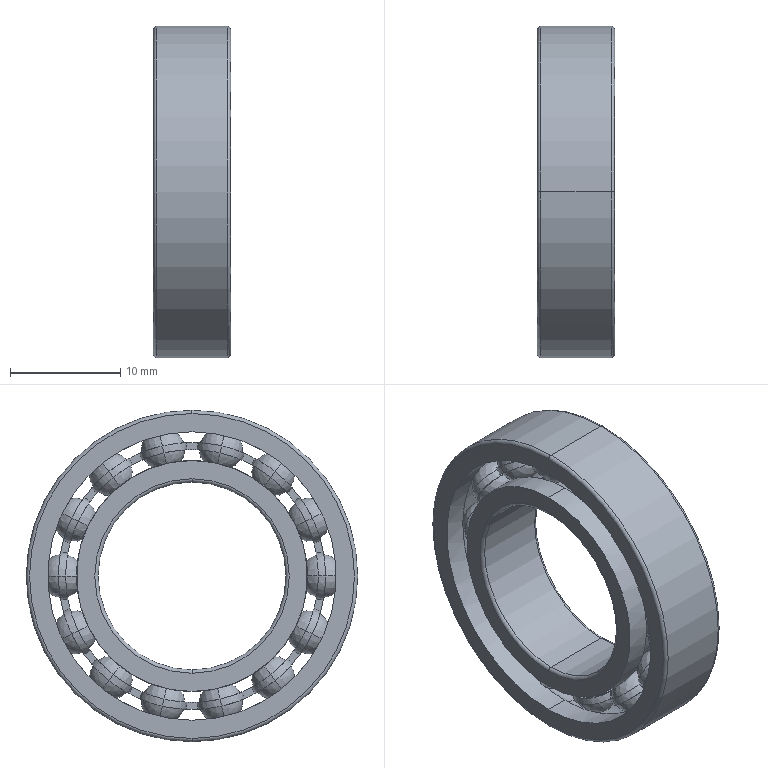Part | SolidWorks | features Revolution 6, Attribute 3, CirPattern 2, RevCut 2, RefAxis 1 | 1 solid | 213 faces | box 7 x 30 x 30 mm | volume 2289 mm3 | sphere 112 | torus 53 | plane 32 | cylinder 16 | commonest cylinder face diameters 20.9 x4 26.1 x4 17 x2 22.85 x2 24.15 x2 30 x2